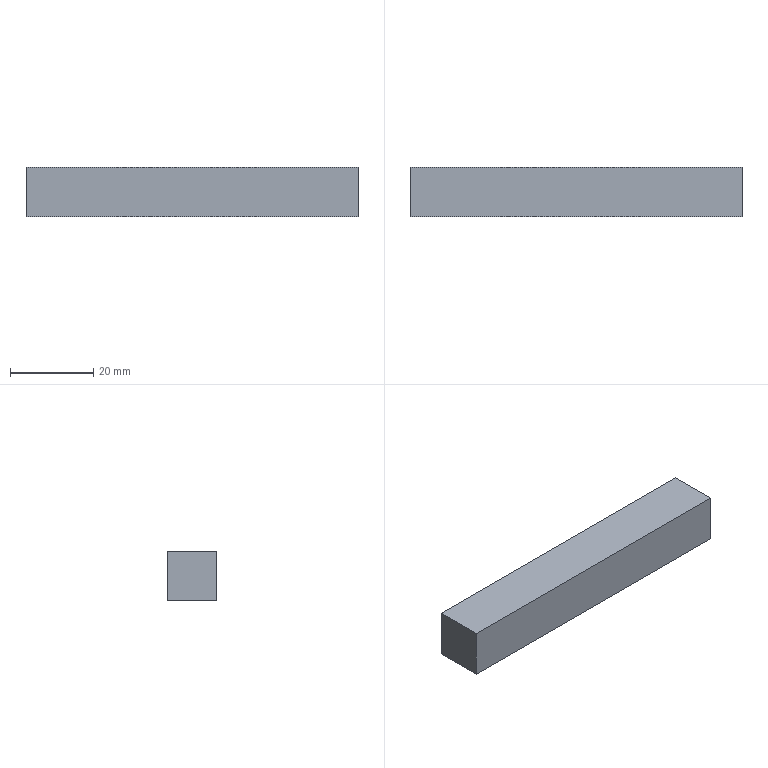Part | STEP file | jiazhi | 1 solid | 6 faces | box 80 x 12 x 12 mm | volume 11520 mm3 | plane 6
STEP:
#1=CARTESIAN_POINT('',(0.,0.,0.));
#2=DIRECTION('',(0.,0.,1.));
#3=DIRECTION('',(1.,0.,0.));
#4=AXIS2_PLACEMENT_3D('',#1,#2,#3);
#5=CARTESIAN_POINT('',(40.,-6.,6.));
#6=VERTEX_POINT('',#5);
#7=CARTESIAN_POINT('',(40.,-6.,-6.));
#8=VERTEX_POINT('',#7);
#9=CARTESIAN_POINT('',(40.,-6.,-6.));
#10=DIRECTION('',(0.,0.,-1.));
#11=VECTOR('',#10,1.);
#12=LINE('',#9,#11);
#13=CARTESIAN_POINT('',(40.,6.,-6.));
#14=DIRECTION('',(-1.,0.,0.));
#15=DIRECTION('',(0.,0.,1.));
#16=AXIS2_PLACEMENT_3D('',#13,#14,#15);
#17=PLANE('',#16);
#18=CARTESIAN_POINT('',(0.,-12.));
#19=DIRECTION('',(-1.,0.));
#20=VECTOR('',#19,1.);
#21=LINE('',#18,#20);
#22=(GEOMETRIC_REPRESENTATION_CONTEXT(2)PARAMETRIC_REPRESENTATION_CONTEXT()REPRESENTATION_CONTEXT('',''));
#23=DEFINITIONAL_REPRESENTATION('',(#21),#22);
#24=PCURVE('',#17,#23);
#25=CARTESIAN_POINT('',(0.,-6.,0.));
#26=DIRECTION('',(0.,1.,0.));
#27=DIRECTION('',(0.,0.,1.));
#28=AXIS2_PLACEMENT_3D('',#25,#26,#27);
#29=PLANE('',#28);
#30=CARTESIAN_POINT('',(-6.,40.));
#31=DIRECTION('',(-1.,0.));
#32=VECTOR('',#31,1.);
#33=LINE('',#30,#32);
#34=(GEOMETRIC_REPRESENTATION_CONTEXT(2)PARAMETRIC_REPRESENTATION_CONTEXT()REPRESENTATION_CONTEXT('',''));
#35=DEFINITIONAL_REPRESENTATION('',(#33),#34);
#36=PCURVE('',#29,#35);
#37=SURFACE_CURVE('',#12,(#24,#36),.PCURVE_S1.);
#38=EDGE_CURVE('',#6,#8,#37,.T.);
#39=ORIENTED_EDGE('',*,*,#38,.T.);
#40=CARTESIAN_POINT('',(40.,6.,-6.));
#41=VERTEX_POINT('',#40);
#42=CARTESIAN_POINT('',(40.,6.,-6.));
#43=DIRECTION('',(0.,-1.,0.));
#44=VECTOR('',#43,1.);
#45=LINE('',#42,#44);
#46=CARTESIAN_POINT('',(0.,0.));
#47=DIRECTION('',(0.,-1.));
#48=VECTOR('',#47,1.);
#49=LINE('',#46,#48);
#50=(GEOMETRIC_REPRESENTATION_CONTEXT(2)PARAMETRIC_REPRESENTATION_CONTEXT()REPRESENTATION_CONTEXT('',''));
#51=DEFINITIONAL_REPRESENTATION('',(#49),#50);
#52=PCURVE('',#17,#51);
#53=CARTESIAN_POINT('',(-40.,6.,-6.));
#54=DIRECTION('',(0.,0.,1.));
#55=DIRECTION('',(1.,0.,0.));
#56=AXIS2_PLACEMENT_3D('',#53,#54,#55);
#57=PLANE('',#56);
#58=CARTESIAN_POINT('',(80.,0.));
#59=DIRECTION('',(0.,-1.));
#60=VECTOR('',#59,1.);
#61=LINE('',#58,#60);
#62=(GEOMETRIC_REPRESENTATION_CONTEXT(2)PARAMETRIC_REPRESENTATION_CONTEXT()REPRESENTATION_CONTEXT('',''));
#63=DEFINITIONAL_REPRESENTATION('',(#61),#62);
#64=PCURVE('',#57,#63);
#65=SURFACE_CURVE('',#45,(#52,#64),.PCURVE_S1.);
#66=EDGE_CURVE('',#41,#8,#65,.T.);
#67=ORIENTED_EDGE('',*,*,#66,.F.);
#68=CARTESIAN_POINT('',(40.,6.,6.));
#69=VERTEX_POINT('',#68);
#70=CARTESIAN_POINT('',(40.,6.,-6.));
#71=DIRECTION('',(0.,0.,-1.));
#72=VECTOR('',#71,1.);
#73=LINE('',#70,#72);
#74=CARTESIAN_POINT('',(0.,0.));
#75=DIRECTION('',(-1.,0.));
#76=VECTOR('',#75,1.);
#77=LINE('',#74,#76);
#78=(GEOMETRIC_REPRESENTATION_CONTEXT(2)PARAMETRIC_REPRESENTATION_CONTEXT()REPRESENTATION_CONTEXT('',''));
#79=DEFINITIONAL_REPRESENTATION('',(#77),#78);
#80=PCURVE('',#17,#79);
#81=CARTESIAN_POINT('',(0.,6.,0.));
#82=DIRECTION('',(0.,1.,0.));
#83=DIRECTION('',(0.,0.,1.));
#84=AXIS2_PLACEMENT_3D('',#81,#82,#83);
#85=PLANE('',#84);
#86=CARTESIAN_POINT('',(-6.,40.));
#87=DIRECTION('',(-1.,0.));
#88=VECTOR('',#87,1.);
#89=LINE('',#86,#88);
#90=(GEOMETRIC_REPRESENTATION_CONTEXT(2)PARAMETRIC_REPRESENTATION_CONTEXT()REPRESENTATION_CONTEXT('',''));
#91=DEFINITIONAL_REPRESENTATION('',(#89),#90);
#92=PCURVE('',#85,#91);
#93=SURFACE_CURVE('',#73,(#80,#92),.PCURVE_S1.);
#94=EDGE_CURVE('',#69,#41,#93,.T.);
#95=ORIENTED_EDGE('',*,*,#94,.F.);
#96=CARTESIAN_POINT('',(40.,6.,6.));
#97=DIRECTION('',(0.,-1.,0.));
#98=VECTOR('',#97,1.);
#99=LINE('',#96,#98);
#100=CARTESIAN_POINT('',(12.,0.));
#101=DIRECTION('',(0.,-1.));
#102=VECTOR('',#101,1.);
#103=LINE('',#100,#102);
#104=(GEOMETRIC_REPRESENTATION_CONTEXT(2)PARAMETRIC_REPRESENTATION_CONTEXT()REPRESENTATION_CONTEXT('',''));
#105=DEFINITIONAL_REPRESENTATION('',(#103),#104);
#106=PCURVE('',#17,#105);
#107=CARTESIAN_POINT('',(-40.,6.,6.));
#108=DIRECTION('',(0.,0.,-1.));
#109=DIRECTION('',(-1.,0.,0.));
#110=AXIS2_PLACEMENT_3D('',#107,#108,#109);
#111=PLANE('',#110);
#112=CARTESIAN_POINT('',(-80.,0.));
#113=DIRECTION('',(0.,-1.));
#114=VECTOR('',#113,1.);
#115=LINE('',#112,#114);
#116=(GEOMETRIC_REPRESENTATION_CONTEXT(2)PARAMETRIC_REPRESENTATION_CONTEXT()REPRESENTATION_CONTEXT('',''));
#117=DEFINITIONAL_REPRESENTATION('',(#115),#116);
#118=PCURVE('',#111,#117);
#119=SURFACE_CURVE('',#99,(#106,#118),.PCURVE_S1.);
#120=EDGE_CURVE('',#69,#6,#119,.T.);
#121=ORIENTED_EDGE('',*,*,#120,.T.);
#122=EDGE_LOOP('',(#39,#67,#95,#121));
#123=FACE_BOUND('',#122,.T.);
#124=ADVANCED_FACE('',(#123),#17,.F.);
#125=CARTESIAN_POINT('',(-40.,-6.,-6.));
#126=VERTEX_POINT('',#125);
#127=CARTESIAN_POINT('',(-40.,-6.,-6.));
#128=DIRECTION('',(-1.,0.,0.));
#129=VECTOR('',#128,1.);
#130=LINE('',#127,#129);
#131=CARTESIAN_POINT('',(0.,-12.));
#132=DIRECTION('',(-1.,0.));
#133=VECTOR('',#132,1.);
#134=LINE('',#131,#133);
#135=(GEOMETRIC_REPRESENTATION_CONTEXT(2)PARAMETRIC_REPRESENTATION_CONTEXT()REPRESENTATION_CONTEXT('',''));
#136=DEFINITIONAL_REPRESENTATION('',(#134),#135);
#137=PCURVE('',#57,#136);
#138=CARTESIAN_POINT('',(-6.,-40.));
#139=DIRECTION('',(0.,-1.));
#140=VECTOR('',#139,1.);
#141=LINE('',#138,#140);
#142=(GEOMETRIC_REPRESENTATION_CONTEXT(2)PARAMETRIC_REPRESENTATION_CONTEXT()REPRESENTATION_CONTEXT('',''));
#143=DEFINITIONAL_REPRESENTATION('',(#141),#142);
#144=PCURVE('',#29,#143);
#145=SURFACE_CURVE('',#130,(#137,#144),.PCURVE_S1.);
#146=EDGE_CURVE('',#8,#126,#145,.T.);
#147=ORIENTED_EDGE('',*,*,#146,.T.);
#148=CARTESIAN_POINT('',(-40.,6.,-6.));
#149=VERTEX_POINT('',#148);
#150=CARTESIAN_POINT('',(-40.,6.,-6.));
#151=DIRECTION('',(0.,-1.,0.));
#152=VECTOR('',#151,1.);
#153=LINE('',#150,#152);
#154=CARTESIAN_POINT('',(0.,0.));
#155=DIRECTION('',(0.,-1.));
#156=VECTOR('',#155,1.);
#157=LINE('',#154,#156);
#158=(GEOMETRIC_REPRESENTATION_CONTEXT(2)PARAMETRIC_REPRESENTATION_CONTEXT()REPRESENTATION_CONTEXT('',''));
#159=DEFINITIONAL_REPRESENTATION('',(#157),#158);
#160=PCURVE('',#57,#159);
#161=CARTESIAN_POINT('',(-40.,6.,-6.));
#162=DIRECTION('',(1.,0.,0.));
#163=DIRECTION('',(0.,0.,-1.));
#164=AXIS2_PLACEMENT_3D('',#161,#162,#163);
#165=PLANE('',#164);
#166=CARTESIAN_POINT('',(0.,0.));
#167=DIRECTION('',(0.,-1.));
#168=VECTOR('',#167,1.);
#169=LINE('',#166,#168);
#170=(GEOMETRIC_REPRESENTATION_CONTEXT(2)PARAMETRIC_REPRESENTATION_CONTEXT()REPRESENTATION_CONTEXT('',''));
#171=DEFINITIONAL_REPRESENTATION('',(#169),#170);
#172=PCURVE('',#165,#171);
#173=SURFACE_CURVE('',#153,(#160,#172),.PCURVE_S1.);
#174=EDGE_CURVE('',#149,#126,#173,.T.);
#175=ORIENTED_EDGE('',*,*,#174,.F.);
#176=CARTESIAN_POINT('',(-40.,6.,-6.));
#177=DIRECTION('',(-1.,0.,0.));
#178=VECTOR('',#177,1.);
#179=LINE('',#176,#178);
#180=CARTESIAN_POINT('',(0.,0.));
#181=DIRECTION('',(-1.,0.));
#182=VECTOR('',#181,1.);
#183=LINE('',#180,#182);
#184=(GEOMETRIC_REPRESENTATION_CONTEXT(2)PARAMETRIC_REPRESENTATION_CONTEXT()REPRESENTATION_CONTEXT('',''));
#185=DEFINITIONAL_REPRESENTATION('',(#183),#184);
#186=PCURVE('',#57,#185);
#187=CARTESIAN_POINT('',(-6.,-40.));
#188=DIRECTION('',(0.,-1.));
#189=VECTOR('',#188,1.);
#190=LINE('',#187,#189);
#191=(GEOMETRIC_REPRESENTATION_CONTEXT(2)PARAMETRIC_REPRESENTATION_CONTEXT()REPRESENTATION_CONTEXT('',''));
#192=DEFINITIONAL_REPRESENTATION('',(#190),#191);
#193=PCURVE('',#85,#192);
#194=SURFACE_CURVE('',#179,(#186,#193),.PCURVE_S1.);
#195=EDGE_CURVE('',#41,#149,#194,.T.);
#196=ORIENTED_EDGE('',*,*,#195,.F.);
#197=ORIENTED_EDGE('',*,*,#66,.T.);
#198=EDGE_LOOP('',(#147,#175,#196,#197));
#199=FACE_BOUND('',#198,.T.);
#200=ADVANCED_FACE('',(#199),#57,.F.);
#201=CARTESIAN_POINT('',(-40.,-6.,6.));
#202=VERTEX_POINT('',#201);
#203=CARTESIAN_POINT('',(-40.,-6.,-6.));
#204=DIRECTION('',(0.,0.,1.));
#205=VECTOR('',#204,1.);
#206=LINE('',#203,#205);
#207=CARTESIAN_POINT('',(0.,-12.));
#208=DIRECTION('',(-1.,0.));
#209=VECTOR('',#208,1.);
#210=LINE('',#207,#209);
#211=(GEOMETRIC_REPRESENTATION_CONTEXT(2)PARAMETRIC_REPRESENTATION_CONTEXT()REPRESENTATION_CONTEXT('',''));
#212=DEFINITIONAL_REPRESENTATION('',(#210),#211);
#213=PCURVE('',#165,#212);
#214=CARTESIAN_POINT('',(-6.,-40.));
#215=DIRECTION('',(1.,0.));
#216=VECTOR('',#215,1.);
#217=LINE('',#214,#216);
#218=(GEOMETRIC_REPRESENTATION_CONTEXT(2)PARAMETRIC_REPRESENTATION_CONTEXT()REPRESENTATION_CONTEXT('',''));
#219=DEFINITIONAL_REPRESENTATION('',(#217),#218);
#220=PCURVE('',#29,#219);
#221=SURFACE_CURVE('',#206,(#213,#220),.PCURVE_S1.);
#222=EDGE_CURVE('',#126,#202,#221,.T.);
#223=ORIENTED_EDGE('',*,*,#222,.T.);
#224=CARTESIAN_POINT('',(-40.,6.,6.));
#225=VERTEX_POINT('',#224);
#226=CARTESIAN_POINT('',(-40.,6.,6.));
#227=DIRECTION('',(0.,-1.,0.));
#228=VECTOR('',#227,1.);
#229=LINE('',#226,#228);
#230=CARTESIAN_POINT('',(-12.,0.));
#231=DIRECTION('',(0.,-1.));
#232=VECTOR('',#231,1.);
#233=LINE('',#230,#232);
#234=(GEOMETRIC_REPRESENTATION_CONTEXT(2)PARAMETRIC_REPRESENTATION_CONTEXT()REPRESENTATION_CONTEXT('',''));
#235=DEFINITIONAL_REPRESENTATION('',(#233),#234);
#236=PCURVE('',#165,#235);
#237=CARTESIAN_POINT('',(0.,0.));
#238=DIRECTION('',(0.,-1.));
#239=VECTOR('',#238,1.);
#240=LINE('',#237,#239);
#241=(GEOMETRIC_REPRESENTATION_CONTEXT(2)PARAMETRIC_REPRESENTATION_CONTEXT()REPRESENTATION_CONTEXT('',''));
#242=DEFINITIONAL_REPRESENTATION('',(#240),#241);
#243=PCURVE('',#111,#242);
#244=SURFACE_CURVE('',#229,(#236,#243),.PCURVE_S1.);
#245=EDGE_CURVE('',#225,#202,#244,.T.);
#246=ORIENTED_EDGE('',*,*,#245,.F.);
#247=CARTESIAN_POINT('',(-40.,6.,-6.));
#248=DIRECTION('',(0.,0.,1.));
#249=VECTOR('',#248,1.);
#250=LINE('',#247,#249);
#251=CARTESIAN_POINT('',(0.,0.));
#252=DIRECTION('',(-1.,0.));
#253=VECTOR('',#252,1.);
#254=LINE('',#251,#253);
#255=(GEOMETRIC_REPRESENTATION_CONTEXT(2)PARAMETRIC_REPRESENTATION_CONTEXT()REPRESENTATION_CONTEXT('',''));
#256=DEFINITIONAL_REPRESENTATION('',(#254),#255);
#257=PCURVE('',#165,#256);
#258=CARTESIAN_POINT('',(-6.,-40.));
#259=DIRECTION('',(1.,0.));
#260=VECTOR('',#259,1.);
#261=LINE('',#258,#260);
#262=(GEOMETRIC_REPRESENTATION_CONTEXT(2)PARAMETRIC_REPRESENTATION_CONTEXT()REPRESENTATION_CONTEXT('',''));
#263=DEFINITIONAL_REPRESENTATION('',(#261),#262);
#264=PCURVE('',#85,#263);
#265=SURFACE_CURVE('',#250,(#257,#264),.PCURVE_S1.);
#266=EDGE_CURVE('',#149,#225,#265,.T.);
#267=ORIENTED_EDGE('',*,*,#266,.F.);
#268=ORIENTED_EDGE('',*,*,#174,.T.);
#269=EDGE_LOOP('',(#223,#246,#267,#268));
#270=FACE_BOUND('',#269,.T.);
#271=ADVANCED_FACE('',(#270),#165,.F.);
#272=CARTESIAN_POINT('',(-40.,-6.,6.));
#273=DIRECTION('',(1.,0.,0.));
#274=VECTOR('',#273,1.);
#275=LINE('',#272,#274);
#276=CARTESIAN_POINT('',(0.,-12.));
#277=DIRECTION('',(-1.,0.));
#278=VECTOR('',#277,1.);
#279=LINE('',#276,#278);
#280=(GEOMETRIC_REPRESENTATION_CONTEXT(2)PARAMETRIC_REPRESENTATION_CONTEXT()REPRESENTATION_CONTEXT('',''));
#281=DEFINITIONAL_REPRESENTATION('',(#279),#280);
#282=PCURVE('',#111,#281);
#283=CARTESIAN_POINT('',(6.,-40.));
#284=DIRECTION('',(0.,1.));
#285=VECTOR('',#284,1.);
#286=LINE('',#283,#285);
#287=(GEOMETRIC_REPRESENTATION_CONTEXT(2)PARAMETRIC_REPRESENTATION_CONTEXT()REPRESENTATION_CONTEXT('',''));
#288=DEFINITIONAL_REPRESENTATION('',(#286),#287);
#289=PCURVE('',#29,#288);
#290=SURFACE_CURVE('',#275,(#282,#289),.PCURVE_S1.);
#291=EDGE_CURVE('',#202,#6,#290,.T.);
#292=ORIENTED_EDGE('',*,*,#291,.T.);
#293=ORIENTED_EDGE('',*,*,#120,.F.);
#294=CARTESIAN_POINT('',(-40.,6.,6.));
#295=DIRECTION('',(1.,0.,0.));
#296=VECTOR('',#295,1.);
#297=LINE('',#294,#296);
#298=CARTESIAN_POINT('',(0.,0.));
#299=DIRECTION('',(-1.,0.));
#300=VECTOR('',#299,1.);
#301=LINE('',#298,#300);
#302=(GEOMETRIC_REPRESENTATION_CONTEXT(2)PARAMETRIC_REPRESENTATION_CONTEXT()REPRESENTATION_CONTEXT('',''));
#303=DEFINITIONAL_REPRESENTATION('',(#301),#302);
#304=PCURVE('',#111,#303);
#305=CARTESIAN_POINT('',(6.,-40.));
#306=DIRECTION('',(0.,1.));
#307=VECTOR('',#306,1.);
#308=LINE('',#305,#307);
#309=(GEOMETRIC_REPRESENTATION_CONTEXT(2)PARAMETRIC_REPRESENTATION_CONTEXT()REPRESENTATION_CONTEXT('',''));
#310=DEFINITIONAL_REPRESENTATION('',(#308),#309);
#311=PCURVE('',#85,#310);
#312=SURFACE_CURVE('',#297,(#304,#311),.PCURVE_S1.);
#313=EDGE_CURVE('',#225,#69,#312,.T.);
#314=ORIENTED_EDGE('',*,*,#313,.F.);
#315=ORIENTED_EDGE('',*,*,#245,.T.);
#316=EDGE_LOOP('',(#292,#293,#314,#315));
#317=FACE_BOUND('',#316,.T.);
#318=ADVANCED_FACE('',(#317),#111,.F.);
#319=ORIENTED_EDGE('',*,*,#94,.T.);
#320=ORIENTED_EDGE('',*,*,#195,.T.);
#321=ORIENTED_EDGE('',*,*,#266,.T.);
#322=ORIENTED_EDGE('',*,*,#313,.T.);
#323=EDGE_LOOP('',(#319,#320,#321,#322));
#324=FACE_BOUND('',#323,.T.);
#325=ADVANCED_FACE('',(#324),#85,.T.);
#326=ORIENTED_EDGE('',*,*,#38,.F.);
#327=ORIENTED_EDGE('',*,*,#291,.F.);
#328=ORIENTED_EDGE('',*,*,#222,.F.);
#329=ORIENTED_EDGE('',*,*,#146,.F.);
#330=EDGE_LOOP('',(#326,#327,#328,#329));
#331=FACE_BOUND('',#330,.T.);
#332=ADVANCED_FACE('',(#331),#29,.F.);
#333=CLOSED_SHELL('',(#124,#200,#271,#318,#325,#332));
#334=MANIFOLD_SOLID_BREP('',#333);
#335=(LENGTH_UNIT()NAMED_UNIT(*)SI_UNIT(.MILLI.,.METRE.));
#336=UNCERTAINTY_MEASURE_WITH_UNIT(LENGTH_MEASURE(0.0000001),#335,'','');
#337=(NAMED_UNIT(*)PLANE_ANGLE_UNIT()SI_UNIT($,.RADIAN.));
#338=(NAMED_UNIT(*)SI_UNIT($,.STERADIAN.)SOLID_ANGLE_UNIT());
#339=(GEOMETRIC_REPRESENTATION_CONTEXT(3)GLOBAL_UNCERTAINTY_ASSIGNED_CONTEXT((#336))GLOBAL_UNIT_ASSIGNED_CONTEXT((#335,#337,#338))REPRESENTATION_CONTEXT('',''));
#340=ADVANCED_BREP_SHAPE_REPRESENTATION('',(#4,#334),#339);